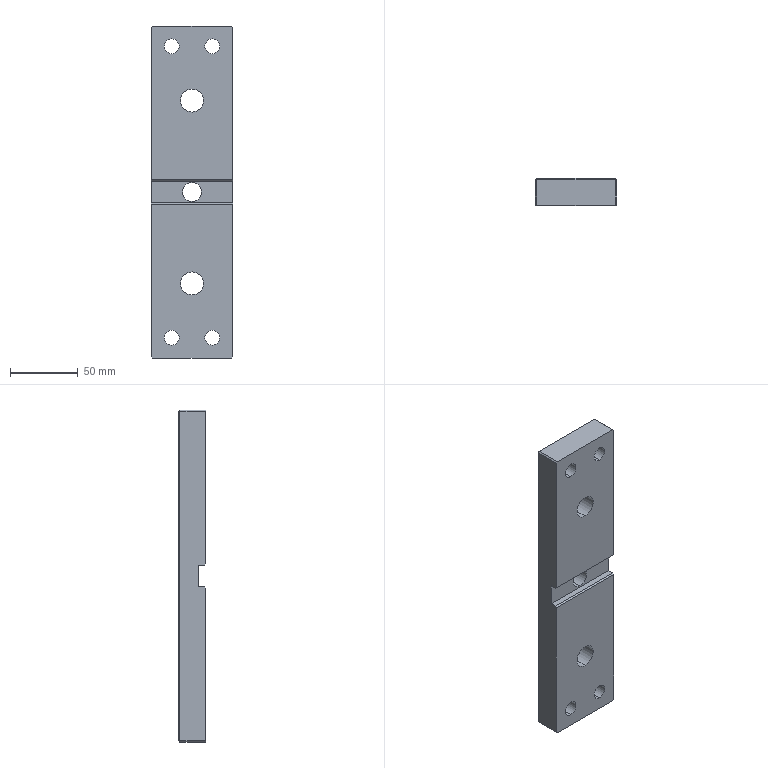Part | SolidWorks | features BaseBody 1 | 1 solid | 46 faces | box 60 x 20 x 245 mm | volume 258955 mm3 | plane 22 | cylinder 18 | cone 6 | commonest cylinder face diameters 11 x8 17 x4 40 x4 14 x2
STEP:
#1=CARTESIAN_POINT('',(15.,-10.,-113.));
#2=VERTEX_POINT('',#1);
#3=CARTESIAN_POINT('',(15.,-10.,-102.));
#4=VERTEX_POINT('',#3);
#5=CARTESIAN_POINT('',(15.,-10.,-107.5));
#6=DIRECTION('',(0.,1.,0.));
#7=DIRECTION('',(0.,0.,1.));
#8=AXIS2_PLACEMENT_3D('',#5,#6,#7);
#9=CIRCLE('',#8,5.5);
#10=EDGE_CURVE('',#2,#4,#9,.T.);
#11=ORIENTED_EDGE('',*,*,#10,.F.);
#12=CARTESIAN_POINT('',(15.,10.,-113.));
#13=VERTEX_POINT('',#12);
#14=CARTESIAN_POINT('',(15.,-10.,-113.));
#15=DIRECTION('',(0.,1.,0.));
#16=VECTOR('',#15,1000.);
#17=LINE('',#14,#16);
#18=EDGE_CURVE('',#2,#13,#17,.T.);
#19=ORIENTED_EDGE('',*,*,#18,.T.);
#20=CARTESIAN_POINT('',(15.,10.,-102.));
#21=VERTEX_POINT('',#20);
#22=CARTESIAN_POINT('',(15.,10.,-107.5));
#23=DIRECTION('',(0.,1.,0.));
#24=DIRECTION('',(0.,0.,1.));
#25=AXIS2_PLACEMENT_3D('',#22,#23,#24);
#26=CIRCLE('',#25,5.5);
#27=EDGE_CURVE('',#13,#21,#26,.T.);
#28=ORIENTED_EDGE('',*,*,#27,.T.);
#29=CARTESIAN_POINT('',(15.,-10.,-102.));
#30=DIRECTION('',(0.,1.,0.));
#31=VECTOR('',#30,1000.);
#32=LINE('',#29,#31);
#33=EDGE_CURVE('',#4,#21,#32,.T.);
#34=ORIENTED_EDGE('',*,*,#33,.F.);
#35=EDGE_LOOP('',(#11,#19,#28,#34));
#36=FACE_OUTER_BOUND('',#35,.T.);
#37=CARTESIAN_POINT('',(15.,-10.,-107.5));
#38=DIRECTION('',(0.,1.,0.));
#39=DIRECTION('',(0.,0.,1.));
#40=AXIS2_PLACEMENT_3D('',#37,#38,#39);
#41=CYLINDRICAL_SURFACE('',#40,5.5);
#42=ADVANCED_FACE('',(#36),#41,.F.);
#43=CARTESIAN_POINT('',(-15.,-10.,-113.));
#44=VERTEX_POINT('',#43);
#45=CARTESIAN_POINT('',(-15.,-10.,-102.));
#46=VERTEX_POINT('',#45);
#47=CARTESIAN_POINT('',(-15.,-10.,-107.5));
#48=DIRECTION('',(0.,1.,0.));
#49=DIRECTION('',(0.,0.,1.));
#50=AXIS2_PLACEMENT_3D('',#47,#48,#49);
#51=CIRCLE('',#50,5.5);
#52=EDGE_CURVE('',#44,#46,#51,.T.);
#53=ORIENTED_EDGE('',*,*,#52,.F.);
#54=CARTESIAN_POINT('',(-15.,10.,-113.));
#55=VERTEX_POINT('',#54);
#56=CARTESIAN_POINT('',(-15.,-10.,-113.));
#57=DIRECTION('',(0.,1.,0.));
#58=VECTOR('',#57,1000.);
#59=LINE('',#56,#58);
#60=EDGE_CURVE('',#44,#55,#59,.T.);
#61=ORIENTED_EDGE('',*,*,#60,.T.);
#62=CARTESIAN_POINT('',(-15.,10.,-102.));
#63=VERTEX_POINT('',#62);
#64=CARTESIAN_POINT('',(-15.,10.,-107.5));
#65=DIRECTION('',(0.,1.,0.));
#66=DIRECTION('',(0.,0.,1.));
#67=AXIS2_PLACEMENT_3D('',#64,#65,#66);
#68=CIRCLE('',#67,5.5);
#69=EDGE_CURVE('',#55,#63,#68,.T.);
#70=ORIENTED_EDGE('',*,*,#69,.T.);
#71=CARTESIAN_POINT('',(-15.,-10.,-102.));
#72=DIRECTION('',(0.,1.,0.));
#73=VECTOR('',#72,1000.);
#74=LINE('',#71,#73);
#75=EDGE_CURVE('',#46,#63,#74,.T.);
#76=ORIENTED_EDGE('',*,*,#75,.F.);
#77=EDGE_LOOP('',(#53,#61,#70,#76));
#78=FACE_OUTER_BOUND('',#77,.T.);
#79=CARTESIAN_POINT('',(-15.,-10.,-107.5));
#80=DIRECTION('',(0.,1.,0.));
#81=DIRECTION('',(0.,0.,1.));
#82=AXIS2_PLACEMENT_3D('',#79,#80,#81);
#83=CYLINDRICAL_SURFACE('',#82,5.5);
#84=ADVANCED_FACE('',(#78),#83,.F.);
#85=CARTESIAN_POINT('',(-15.,-10.,102.));
#86=VERTEX_POINT('',#85);
#87=CARTESIAN_POINT('',(-15.,-10.,113.));
#88=VERTEX_POINT('',#87);
#89=CARTESIAN_POINT('',(-15.,-10.,107.5));
#90=DIRECTION('',(0.,1.,0.));
#91=DIRECTION('',(0.,0.,1.));
#92=AXIS2_PLACEMENT_3D('',#89,#90,#91);
#93=CIRCLE('',#92,5.5);
#94=EDGE_CURVE('',#86,#88,#93,.T.);
#95=ORIENTED_EDGE('',*,*,#94,.F.);
#96=CARTESIAN_POINT('',(-15.,10.,102.));
#97=VERTEX_POINT('',#96);
#98=CARTESIAN_POINT('',(-15.,-10.,102.));
#99=DIRECTION('',(0.,1.,0.));
#100=VECTOR('',#99,1000.);
#101=LINE('',#98,#100);
#102=EDGE_CURVE('',#86,#97,#101,.T.);
#103=ORIENTED_EDGE('',*,*,#102,.T.);
#104=CARTESIAN_POINT('',(-15.,10.,113.));
#105=VERTEX_POINT('',#104);
#106=CARTESIAN_POINT('',(-15.,10.,107.5));
#107=DIRECTION('',(0.,1.,0.));
#108=DIRECTION('',(0.,0.,1.));
#109=AXIS2_PLACEMENT_3D('',#106,#107,#108);
#110=CIRCLE('',#109,5.5);
#111=EDGE_CURVE('',#97,#105,#110,.T.);
#112=ORIENTED_EDGE('',*,*,#111,.T.);
#113=CARTESIAN_POINT('',(-15.,-10.,113.));
#114=DIRECTION('',(0.,1.,0.));
#115=VECTOR('',#114,1000.);
#116=LINE('',#113,#115);
#117=EDGE_CURVE('',#88,#105,#116,.T.);
#118=ORIENTED_EDGE('',*,*,#117,.F.);
#119=EDGE_LOOP('',(#95,#103,#112,#118));
#120=FACE_OUTER_BOUND('',#119,.T.);
#121=CARTESIAN_POINT('',(-15.,-10.,107.5));
#122=DIRECTION('',(0.,1.,0.));
#123=DIRECTION('',(0.,0.,1.));
#124=AXIS2_PLACEMENT_3D('',#121,#122,#123);
#125=CYLINDRICAL_SURFACE('',#124,5.5);
#126=ADVANCED_FACE('',(#120),#125,.F.);
#127=CARTESIAN_POINT('',(15.,-10.,102.));
#128=VERTEX_POINT('',#127);
#129=CARTESIAN_POINT('',(15.,-10.,113.));
#130=VERTEX_POINT('',#129);
#131=CARTESIAN_POINT('',(15.,-10.,107.5));
#132=DIRECTION('',(0.,1.,0.));
#133=DIRECTION('',(0.,0.,1.));
#134=AXIS2_PLACEMENT_3D('',#131,#132,#133);
#135=CIRCLE('',#134,5.5);
#136=EDGE_CURVE('',#128,#130,#135,.T.);
#137=ORIENTED_EDGE('',*,*,#136,.F.);
#138=CARTESIAN_POINT('',(15.,10.,102.));
#139=VERTEX_POINT('',#138);
#140=CARTESIAN_POINT('',(15.,-10.,102.));
#141=DIRECTION('',(0.,1.,0.));
#142=VECTOR('',#141,1000.);
#143=LINE('',#140,#142);
#144=EDGE_CURVE('',#128,#139,#143,.T.);
#145=ORIENTED_EDGE('',*,*,#144,.T.);
#146=CARTESIAN_POINT('',(15.,10.,113.));
#147=VERTEX_POINT('',#146);
#148=CARTESIAN_POINT('',(15.,10.,107.5));
#149=DIRECTION('',(0.,1.,0.));
#150=DIRECTION('',(0.,0.,1.));
#151=AXIS2_PLACEMENT_3D('',#148,#149,#150);
#152=CIRCLE('',#151,5.5);
#153=EDGE_CURVE('',#139,#147,#152,.T.);
#154=ORIENTED_EDGE('',*,*,#153,.T.);
#155=CARTESIAN_POINT('',(15.,-10.,113.));
#156=DIRECTION('',(0.,1.,0.));
#157=VECTOR('',#156,1000.);
#158=LINE('',#155,#157);
#159=EDGE_CURVE('',#130,#147,#158,.T.);
#160=ORIENTED_EDGE('',*,*,#159,.F.);
#161=EDGE_LOOP('',(#137,#145,#154,#160));
#162=FACE_OUTER_BOUND('',#161,.T.);
#163=CARTESIAN_POINT('',(15.,-10.,107.5));
#164=DIRECTION('',(0.,1.,0.));
#165=DIRECTION('',(0.,0.,1.));
#166=AXIS2_PLACEMENT_3D('',#163,#164,#165);
#167=CYLINDRICAL_SURFACE('',#166,5.5);
#168=ADVANCED_FACE('',(#162),#167,.F.);
#169=CARTESIAN_POINT('',(0.,9.,-87.5));
#170=VERTEX_POINT('',#169);
#171=CARTESIAN_POINT('',(0.,9.,-47.5));
#172=VERTEX_POINT('',#171);
#173=CARTESIAN_POINT('',(0.,9.,-67.5));
#174=DIRECTION('',(0.,1.,0.));
#175=DIRECTION('',(0.,0.,-1.));
#176=AXIS2_PLACEMENT_3D('',#173,#174,#175);
#177=CIRCLE('',#176,20.);
#178=EDGE_CURVE('',#170,#172,#177,.T.);
#179=ORIENTED_EDGE('',*,*,#178,.F.);
#180=CARTESIAN_POINT('',(0.,10.,-88.5));
#181=VERTEX_POINT('',#180);
#182=CARTESIAN_POINT('',(0.,10.,-88.5));
#183=DIRECTION('',(0.,0.7071,-0.7071));
#184=VECTOR('',#183,1000.);
#185=LINE('',#182,#184);
#186=EDGE_CURVE('',#170,#181,#185,.T.);
#187=ORIENTED_EDGE('',*,*,#186,.T.);
#188=CARTESIAN_POINT('',(0.,10.,-46.5));
#189=VERTEX_POINT('',#188);
#190=CARTESIAN_POINT('',(0.,10.,-67.5));
#191=DIRECTION('',(0.,-1.,0.));
#192=DIRECTION('',(0.,0.,-1.));
#193=AXIS2_PLACEMENT_3D('',#190,#191,#192);
#194=CIRCLE('',#193,21.);
#195=EDGE_CURVE('',#189,#181,#194,.T.);
#196=ORIENTED_EDGE('',*,*,#195,.F.);
#197=CARTESIAN_POINT('',(0.,10.,-46.5));
#198=DIRECTION('',(0.,0.7071,0.7071));
#199=VECTOR('',#198,1000.);
#200=LINE('',#197,#199);
#201=EDGE_CURVE('',#172,#189,#200,.T.);
#202=ORIENTED_EDGE('',*,*,#201,.F.);
#203=EDGE_LOOP('',(#179,#187,#196,#202));
#204=FACE_OUTER_BOUND('',#203,.T.);
#205=CARTESIAN_POINT('',(0.,10.,-67.5));
#206=DIRECTION('',(0.,1.,0.));
#207=DIRECTION('',(0.,0.,1.));
#208=AXIS2_PLACEMENT_3D('',#205,#206,#207);
#209=CONICAL_SURFACE('',#208,21.,0.7854);
#210=ADVANCED_FACE('',(#204),#209,.F.);
#211=CARTESIAN_POINT('',(0.,9.,47.5));
#212=VERTEX_POINT('',#211);
#213=CARTESIAN_POINT('',(0.,9.,87.5));
#214=VERTEX_POINT('',#213);
#215=CARTESIAN_POINT('',(0.,9.,67.5));
#216=DIRECTION('',(0.,1.,0.));
#217=DIRECTION('',(0.,0.,-1.));
#218=AXIS2_PLACEMENT_3D('',#215,#216,#217);
#219=CIRCLE('',#218,20.);
#220=EDGE_CURVE('',#212,#214,#219,.T.);
#221=ORIENTED_EDGE('',*,*,#220,.F.);
#222=CARTESIAN_POINT('',(0.,10.,46.5));
#223=VERTEX_POINT('',#222);
#224=CARTESIAN_POINT('',(0.,10.,46.5));
#225=DIRECTION('',(0.,0.7071,-0.7071));
#226=VECTOR('',#225,1000.);
#227=LINE('',#224,#226);
#228=EDGE_CURVE('',#212,#223,#227,.T.);
#229=ORIENTED_EDGE('',*,*,#228,.T.);
#230=CARTESIAN_POINT('',(0.,10.,88.5));
#231=VERTEX_POINT('',#230);
#232=CARTESIAN_POINT('',(0.,10.,67.5));
#233=DIRECTION('',(0.,-1.,0.));
#234=DIRECTION('',(0.,0.,-1.));
#235=AXIS2_PLACEMENT_3D('',#232,#233,#234);
#236=CIRCLE('',#235,21.);
#237=EDGE_CURVE('',#231,#223,#236,.T.);
#238=ORIENTED_EDGE('',*,*,#237,.F.);
#239=CARTESIAN_POINT('',(0.,10.,88.5));
#240=DIRECTION('',(0.,0.7071,0.7071));
#241=VECTOR('',#240,1000.);
#242=LINE('',#239,#241);
#243=EDGE_CURVE('',#214,#231,#242,.T.);
#244=ORIENTED_EDGE('',*,*,#243,.F.);
#245=EDGE_LOOP('',(#221,#229,#238,#244));
#246=FACE_OUTER_BOUND('',#245,.T.);
#247=CARTESIAN_POINT('',(0.,10.,67.5));
#248=DIRECTION('',(0.,1.,0.));
#249=DIRECTION('',(0.,0.,1.));
#250=AXIS2_PLACEMENT_3D('',#247,#248,#249);
#251=CONICAL_SURFACE('',#250,21.,0.7854);
#252=ADVANCED_FACE('',(#246),#251,.F.);
#253=CARTESIAN_POINT('',(0.,8.975,-7.));
#254=VERTEX_POINT('',#253);
#255=CARTESIAN_POINT('',(0.,8.975,7.));
#256=VERTEX_POINT('',#255);
#257=CARTESIAN_POINT('',(0.,8.975,0.));
#258=DIRECTION('',(0.,1.,0.));
#259=DIRECTION('',(0.,0.,1.));
#260=AXIS2_PLACEMENT_3D('',#257,#258,#259);
#261=CIRCLE('',#260,7.);
#262=EDGE_CURVE('',#254,#256,#261,.T.);
#263=ORIENTED_EDGE('',*,*,#262,.F.);
#264=CARTESIAN_POINT('',(0.,10.,-8.025));
#265=VERTEX_POINT('',#264);
#266=CARTESIAN_POINT('',(0.,10.,-8.025));
#267=DIRECTION('',(0.,0.7071,-0.7071));
#268=VECTOR('',#267,1000.);
#269=LINE('',#266,#268);
#270=EDGE_CURVE('',#254,#265,#269,.T.);
#271=ORIENTED_EDGE('',*,*,#270,.T.);
#272=CARTESIAN_POINT('',(0.,10.,8.025));
#273=VERTEX_POINT('',#272);
#274=CARTESIAN_POINT('',(0.,10.,0.));
#275=DIRECTION('',(0.,1.,0.));
#276=DIRECTION('',(0.,0.,1.));
#277=AXIS2_PLACEMENT_3D('',#274,#275,#276);
#278=CIRCLE('',#277,8.025);
#279=EDGE_CURVE('',#265,#273,#278,.T.);
#280=ORIENTED_EDGE('',*,*,#279,.T.);
#281=CARTESIAN_POINT('',(0.,10.,8.025));
#282=DIRECTION('',(0.,0.7071,0.7071));
#283=VECTOR('',#282,1000.);
#284=LINE('',#281,#283);
#285=EDGE_CURVE('',#256,#273,#284,.T.);
#286=ORIENTED_EDGE('',*,*,#285,.F.);
#287=EDGE_LOOP('',(#263,#271,#280,#286));
#288=FACE_OUTER_BOUND('',#287,.T.);
#289=CARTESIAN_POINT('',(0.,10.,0.));
#290=DIRECTION('',(0.,1.,0.));
#291=DIRECTION('',(0.,0.,1.));
#292=AXIS2_PLACEMENT_3D('',#289,#290,#291);
#293=CONICAL_SURFACE('',#292,8.025,0.7854);
#294=ADVANCED_FACE('',(#288),#293,.F.);
#295=CARTESIAN_POINT('',(0.,-4.5,7.));
#296=VERTEX_POINT('',#295);
#297=CARTESIAN_POINT('',(0.,-4.5,-7.));
#298=VERTEX_POINT('',#297);
#299=CARTESIAN_POINT('',(0.,-4.5,0.));
#300=DIRECTION('',(0.,-1.,0.));
#301=DIRECTION('',(0.,0.,1.));
#302=AXIS2_PLACEMENT_3D('',#299,#300,#301);
#303=CIRCLE('',#302,7.);
#304=EDGE_CURVE('',#296,#298,#303,.T.);
#305=ORIENTED_EDGE('',*,*,#304,.T.);
#306=CARTESIAN_POINT('',(0.,10.,-7.));
#307=DIRECTION('',(0.,1.,0.));
#308=VECTOR('',#307,1000.);
#309=LINE('',#306,#308);
#310=EDGE_CURVE('',#298,#254,#309,.T.);
#311=ORIENTED_EDGE('',*,*,#310,.T.);
#312=ORIENTED_EDGE('',*,*,#262,.T.);
#313=CARTESIAN_POINT('',(0.,10.,7.));
#314=DIRECTION('',(0.,1.,0.));
#315=VECTOR('',#314,1000.);
#316=LINE('',#313,#315);
#317=EDGE_CURVE('',#296,#256,#316,.T.);
#318=ORIENTED_EDGE('',*,*,#317,.F.);
#319=EDGE_LOOP('',(#305,#311,#312,#318));
#320=FACE_OUTER_BOUND('',#319,.T.);
#321=CARTESIAN_POINT('',(0.,10.,0.));
#322=DIRECTION('',(0.,1.,0.));
#323=DIRECTION('',(0.,0.,1.));
#324=AXIS2_PLACEMENT_3D('',#321,#322,#323);
#325=CYLINDRICAL_SURFACE('',#324,7.);
#326=ADVANCED_FACE('',(#320),#325,.F.);
#327=CARTESIAN_POINT('',(0.,5.,87.5));
#328=VERTEX_POINT('',#327);
#329=CARTESIAN_POINT('',(0.,5.,47.5));
#330=VERTEX_POINT('',#329);
#331=CARTESIAN_POINT('',(0.,5.,67.5));
#332=DIRECTION('',(0.,-1.,0.));
#333=DIRECTION('',(0.,0.,-1.));
#334=AXIS2_PLACEMENT_3D('',#331,#332,#333);
#335=CIRCLE('',#334,20.);
#336=EDGE_CURVE('',#328,#330,#335,.T.);
#337=ORIENTED_EDGE('',*,*,#336,.T.);
#338=CARTESIAN_POINT('',(0.,5.,47.5));
#339=DIRECTION('',(0.,1.,0.));
#340=VECTOR('',#339,1000.);
#341=LINE('',#338,#340);
#342=EDGE_CURVE('',#330,#212,#341,.T.);
#343=ORIENTED_EDGE('',*,*,#342,.T.);
#344=ORIENTED_EDGE('',*,*,#220,.T.);
#345=CARTESIAN_POINT('',(0.,5.,87.5));
#346=DIRECTION('',(0.,1.,0.));
#347=VECTOR('',#346,1000.);
#348=LINE('',#345,#347);
#349=EDGE_CURVE('',#328,#214,#348,.T.);
#350=ORIENTED_EDGE('',*,*,#349,.F.);
#351=EDGE_LOOP('',(#337,#343,#344,#350));
#352=FACE_OUTER_BOUND('',#351,.T.);
#353=CARTESIAN_POINT('',(0.,5.,67.5));
#354=DIRECTION('',(0.,1.,0.));
#355=DIRECTION('',(0.,0.,1.));
#356=AXIS2_PLACEMENT_3D('',#353,#354,#355);
#357=CYLINDRICAL_SURFACE('',#356,20.);
#358=ADVANCED_FACE('',(#352),#357,.F.);
#359=CARTESIAN_POINT('',(0.,5.,-47.5));
#360=VERTEX_POINT('',#359);
#361=CARTESIAN_POINT('',(0.,5.,-87.5));
#362=VERTEX_POINT('',#361);
#363=CARTESIAN_POINT('',(0.,5.,-67.5));
#364=DIRECTION('',(0.,-1.,0.));
#365=DIRECTION('',(0.,0.,-1.));
#366=AXIS2_PLACEMENT_3D('',#363,#364,#365);
#367=CIRCLE('',#366,20.);
#368=EDGE_CURVE('',#360,#362,#367,.T.);
#369=ORIENTED_EDGE('',*,*,#368,.T.);
#370=CARTESIAN_POINT('',(0.,5.,-87.5));
#371=DIRECTION('',(0.,1.,0.));
#372=VECTOR('',#371,1000.);
#373=LINE('',#370,#372);
#374=EDGE_CURVE('',#362,#170,#373,.T.);
#375=ORIENTED_EDGE('',*,*,#374,.T.);
#376=ORIENTED_EDGE('',*,*,#178,.T.);
#377=CARTESIAN_POINT('',(0.,5.,-47.5));
#378=DIRECTION('',(0.,1.,0.));
#379=VECTOR('',#378,1000.);
#380=LINE('',#377,#379);
#381=EDGE_CURVE('',#360,#172,#380,.T.);
#382=ORIENTED_EDGE('',*,*,#381,.F.);
#383=EDGE_LOOP('',(#369,#375,#376,#382));
#384=FACE_OUTER_BOUND('',#383,.T.);
#385=CARTESIAN_POINT('',(0.,5.,-67.5));
#386=DIRECTION('',(0.,1.,0.));
#387=DIRECTION('',(0.,0.,1.));
#388=AXIS2_PLACEMENT_3D('',#385,#386,#387);
#389=CYLINDRICAL_SURFACE('',#388,20.);
#390=ADVANCED_FACE('',(#384),#389,.F.);
#391=CARTESIAN_POINT('',(0.,5.,-59.));
#392=VERTEX_POINT('',#391);
#393=CARTESIAN_POINT('',(0.,5.,-76.));
#394=VERTEX_POINT('',#393);
#395=CARTESIAN_POINT('',(0.,5.,-67.5));
#396=DIRECTION('',(0.,-1.,0.));
#397=DIRECTION('',(0.,0.,-1.));
#398=AXIS2_PLACEMENT_3D('',#395,#396,#397);
#399=CIRCLE('',#398,8.5);
#400=EDGE_CURVE('',#392,#394,#399,.T.);
#401=ORIENTED_EDGE('',*,*,#400,.F.);
#402=CARTESIAN_POINT('',(0.,-10.,-59.));
#403=VERTEX_POINT('',#402);
#404=CARTESIAN_POINT('',(0.,10.,-59.));
#405=DIRECTION('',(0.,-1.,0.));
#406=VECTOR('',#405,1000.);
#407=LINE('',#404,#406);
#408=EDGE_CURVE('',#392,#403,#407,.T.);
#409=ORIENTED_EDGE('',*,*,#408,.T.);
#410=CARTESIAN_POINT('',(0.,-10.,-76.));
#411=VERTEX_POINT('',#410);
#412=CARTESIAN_POINT('',(0.,-10.,-67.5));
#413=DIRECTION('',(0.,1.,0.));
#414=DIRECTION('',(0.,0.,1.));
#415=AXIS2_PLACEMENT_3D('',#412,#413,#414);
#416=CIRCLE('',#415,8.5);
#417=EDGE_CURVE('',#411,#403,#416,.T.);
#418=ORIENTED_EDGE('',*,*,#417,.F.);
#419=CARTESIAN_POINT('',(0.,10.,-76.));
#420=DIRECTION('',(0.,-1.,0.));
#421=VECTOR('',#420,1000.);
#422=LINE('',#419,#421);
#423=EDGE_CURVE('',#394,#411,#422,.T.);
#424=ORIENTED_EDGE('',*,*,#423,.F.);
#425=EDGE_LOOP('',(#401,#409,#418,#424));
#426=FACE_OUTER_BOUND('',#425,.T.);
#427=CARTESIAN_POINT('',(0.,10.,-67.5));
#428=DIRECTION('',(0.,-1.,0.));
#429=DIRECTION('',(0.,0.,-1.));
#430=AXIS2_PLACEMENT_3D('',#427,#428,#429);
#431=CYLINDRICAL_SURFACE('',#430,8.5);
#432=ADVANCED_FACE('',(#426),#431,.F.);
#433=CARTESIAN_POINT('',(0.,5.,76.));
#434=VERTEX_POINT('',#433);
#435=CARTESIAN_POINT('',(0.,5.,59.));
#436=VERTEX_POINT('',#435);
#437=CARTESIAN_POINT('',(0.,5.,67.5));
#438=DIRECTION('',(0.,-1.,0.));
#439=DIRECTION('',(0.,0.,-1.));
#440=AXIS2_PLACEMENT_3D('',#437,#438,#439);
#441=CIRCLE('',#440,8.5);
#442=EDGE_CURVE('',#434,#436,#441,.T.);
#443=ORIENTED_EDGE('',*,*,#442,.F.);
#444=CARTESIAN_POINT('',(0.,-10.,76.));
#445=VERTEX_POINT('',#444);
#446=CARTESIAN_POINT('',(0.,10.,76.));
#447=DIRECTION('',(0.,-1.,0.));
#448=VECTOR('',#447,1000.);
#449=LINE('',#446,#448);
#450=EDGE_CURVE('',#434,#445,#449,.T.);
#451=ORIENTED_EDGE('',*,*,#450,.T.);
#452=CARTESIAN_POINT('',(0.,-10.,59.));
#453=VERTEX_POINT('',#452);
#454=CARTESIAN_POINT('',(0.,-10.,67.5));
#455=DIRECTION('',(0.,1.,0.));
#456=DIRECTION('',(0.,0.,1.));
#457=AXIS2_PLACEMENT_3D('',#454,#455,#456);
#458=CIRCLE('',#457,8.5);
#459=EDGE_CURVE('',#453,#445,#458,.T.);
#460=ORIENTED_EDGE('',*,*,#459,.F.);
#461=CARTESIAN_POINT('',(0.,10.,59.));
#462=DIRECTION('',(0.,-1.,0.));
#463=VECTOR('',#462,1000.);
#464=LINE('',#461,#463);
#465=EDGE_CURVE('',#436,#453,#464,.T.);
#466=ORIENTED_EDGE('',*,*,#465,.F.);
#467=EDGE_LOOP('',(#443,#451,#460,#466));
#468=FACE_OUTER_BOUND('',#467,.T.);
#469=CARTESIAN_POINT('',(0.,10.,67.5));
#470=DIRECTION('',(0.,-1.,0.));
#471=DIRECTION('',(0.,0.,-1.));
#472=AXIS2_PLACEMENT_3D('',#469,#470,#471);
#473=CYLINDRICAL_SURFACE('',#472,8.5);
#474=ADVANCED_FACE('',(#468),#473,.F.);
#475=CARTESIAN_POINT('',(15.,-10.,-107.5));
#476=DIRECTION('',(0.,1.,0.));
#477=DIRECTION('',(0.,0.,1.));
#478=AXIS2_PLACEMENT_3D('',#475,#476,#477);
#479=CIRCLE('',#478,5.5);
#480=EDGE_CURVE('',#4,#2,#479,.T.);
#481=ORIENTED_EDGE('',*,*,#480,.T.);
#482=ORIENTED_EDGE('',*,*,#10,.T.);
#483=EDGE_LOOP('',(#481,#482));
#484=FACE_BOUND('',#483,.T.);
#485=CARTESIAN_POINT('',(-15.,-10.,-107.5));
#486=DIRECTION('',(0.,1.,0.));
#487=DIRECTION('',(0.,0.,1.));
#488=AXIS2_PLACEMENT_3D('',#485,#486,#487);
#489=CIRCLE('',#488,5.5);
#490=EDGE_CURVE('',#46,#44,#489,.T.);
#491=ORIENTED_EDGE('',*,*,#490,.T.);
#492=ORIENTED_EDGE('',*,*,#52,.T.);
#493=EDGE_LOOP('',(#491,#492));
#494=FACE_BOUND('',#493,.T.);
#495=CARTESIAN_POINT('',(30.,-10.,-9.));
#496=VERTEX_POINT('',#495);
#497=CARTESIAN_POINT('',(30.,-10.,-121.5));
#498=VERTEX_POINT('',#497);
#499=CARTESIAN_POINT('',(30.,-10.,-96.5));
#500=DIRECTION('',(0.,0.,-1.));
#501=VECTOR('',#500,1000.);
#502=LINE('',#499,#501);
#503=EDGE_CURVE('',#496,#498,#502,.T.);
#504=ORIENTED_EDGE('',*,*,#503,.F.);
#505=CARTESIAN_POINT('',(-30.,-10.,-9.));
#506=VERTEX_POINT('',#505);
#507=CARTESIAN_POINT('',(-30.,-10.,-9.));
#508=DIRECTION('',(-1.,0.,0.));
#509=VECTOR('',#508,1000.);
#510=LINE('',#507,#509);
#511=EDGE_CURVE('',#496,#506,#510,.T.);
#512=ORIENTED_EDGE('',*,*,#511,.T.);
#513=CARTESIAN_POINT('',(-30.,-10.,-121.5));
#514=VERTEX_POINT('',#513);
#515=CARTESIAN_POINT('',(-30.,-10.,96.5));
#516=DIRECTION('',(0.,0.,1.));
#517=VECTOR('',#516,1000.);
#518=LINE('',#515,#517);
#519=EDGE_CURVE('',#514,#506,#518,.T.);
#520=ORIENTED_EDGE('',*,*,#519,.F.);
#521=CARTESIAN_POINT('',(-29.,-10.,-122.5));
#522=VERTEX_POINT('',#521);
#523=CARTESIAN_POINT('',(-30.,-10.,-121.5));
#524=DIRECTION('',(-0.7071,0.,0.7071));
#525=VECTOR('',#524,1000.);
#526=LINE('',#523,#525);
#527=EDGE_CURVE('',#522,#514,#526,.T.);
#528=ORIENTED_EDGE('',*,*,#527,.F.);
#529=CARTESIAN_POINT('',(29.,-10.,-122.5));
#530=VERTEX_POINT('',#529);
#531=CARTESIAN_POINT('',(-29.,-10.,-122.5));
#532=DIRECTION('',(-1.,0.,0.));
#533=VECTOR('',#532,1000.);
#534=LINE('',#531,#533);
#535=EDGE_CURVE('',#530,#522,#534,.T.);
#536=ORIENTED_EDGE('',*,*,#535,.F.);
#537=CARTESIAN_POINT('',(29.,-10.,-122.5));
#538=DIRECTION('',(-0.7071,0.,-0.7071));
#539=VECTOR('',#538,1000.);
#540=LINE('',#537,#539);
#541=EDGE_CURVE('',#498,#530,#540,.T.);
#542=ORIENTED_EDGE('',*,*,#541,.F.);
#543=EDGE_LOOP('',(#504,#512,#520,#528,#536,#542));
#544=FACE_OUTER_BOUND('',#543,.T.);
#545=ORIENTED_EDGE('',*,*,#417,.T.);
#546=CARTESIAN_POINT('',(0.,-10.,-67.5));
#547=DIRECTION('',(0.,1.,0.));
#548=DIRECTION('',(0.,0.,1.));
#549=AXIS2_PLACEMENT_3D('',#546,#547,#548);
#550=CIRCLE('',#549,8.5);
#551=EDGE_CURVE('',#403,#411,#550,.T.);
#552=ORIENTED_EDGE('',*,*,#551,.T.);
#553=EDGE_LOOP('',(#545,#552));
#554=FACE_BOUND('',#553,.T.);
#555=CARTESIAN_POINT('',(0.,-10.,0.));
#556=DIRECTION('',(0.,-1.,0.));
#557=DIRECTION('',(0.,0.,-1.));
#558=AXIS2_PLACEMENT_3D('',#555,#556,#557);
#559=PLANE('',#558);
#560=ADVANCED_FACE('',(#484,#494,#544,#554),#559,.T.);
#561=CARTESIAN_POINT('',(-15.,10.,107.5));
#562=DIRECTION('',(0.,1.,0.));
#563=DIRECTION('',(0.,0.,1.));
#564=AXIS2_PLACEMENT_3D('',#561,#562,#563);
#565=CIRCLE('',#564,5.5);
#566=EDGE_CURVE('',#105,#97,#565,.T.);
#567=ORIENTED_EDGE('',*,*,#566,.F.);
#568=ORIENTED_EDGE('',*,*,#111,.F.);
#569=EDGE_LOOP('',(#567,#568));
#570=FACE_BOUND('',#569,.T.);
#571=CARTESIAN_POINT('',(15.,10.,107.5));
#572=DIRECTION('',(0.,1.,0.));
#573=DIRECTION('',(0.,0.,1.));
#574=AXIS2_PLACEMENT_3D('',#571,#572,#573);
#575=CIRCLE('',#574,5.5);
#576=EDGE_CURVE('',#147,#139,#575,.T.);
#577=ORIENTED_EDGE('',*,*,#576,.F.);
#578=ORIENTED_EDGE('',*,*,#153,.F.);
#579=EDGE_LOOP('',(#577,#578));
#580=FACE_BOUND('',#579,.T.);
#581=CARTESIAN_POINT('',(15.,10.,-107.5));
#582=DIRECTION('',(0.,1.,0.));
#583=DIRECTION('',(0.,0.,1.));
#584=AXIS2_PLACEMENT_3D('',#581,#582,#583);
#585=CIRCLE('',#584,5.5);
#586=EDGE_CURVE('',#21,#13,#585,.T.);
#587=ORIENTED_EDGE('',*,*,#586,.F.);
#588=ORIENTED_EDGE('',*,*,#27,.F.);
#589=EDGE_LOOP('',(#587,#588));
#590=FACE_BOUND('',#589,.T.);
#591=CARTESIAN_POINT('',(-15.,10.,-107.5));
#592=DIRECTION('',(0.,1.,0.));
#593=DIRECTION('',(0.,0.,1.));
#594=AXIS2_PLACEMENT_3D('',#591,#592,#593);
#595=CIRCLE('',#594,5.5);
#596=EDGE_CURVE('',#63,#55,#595,.T.);
#597=ORIENTED_EDGE('',*,*,#596,.F.);
#598=ORIENTED_EDGE('',*,*,#69,.F.);
#599=EDGE_LOOP('',(#597,#598));
#600=FACE_BOUND('',#599,.T.);
#601=ORIENTED_EDGE('',*,*,#237,.T.);
#602=CARTESIAN_POINT('',(0.,10.,67.5));
#603=DIRECTION('',(0.,-1.,0.));
#604=DIRECTION('',(0.,0.,-1.));
#605=AXIS2_PLACEMENT_3D('',#602,#603,#604);
#606=CIRCLE('',#605,21.);
#607=EDGE_CURVE('',#223,#231,#606,.T.);
#608=ORIENTED_EDGE('',*,*,#607,.T.);
#609=EDGE_LOOP('',(#601,#608));
#610=FACE_BOUND('',#609,.T.);
#611=ORIENTED_EDGE('',*,*,#195,.T.);
#612=CARTESIAN_POINT('',(0.,10.,-67.5));
#613=DIRECTION('',(0.,-1.,0.));
#614=DIRECTION('',(0.,0.,-1.));
#615=AXIS2_PLACEMENT_3D('',#612,#613,#614);
#616=CIRCLE('',#615,21.);
#617=EDGE_CURVE('',#181,#189,#616,.T.);
#618=ORIENTED_EDGE('',*,*,#617,.T.);
#619=EDGE_LOOP('',(#611,#618));
#620=FACE_BOUND('',#619,.T.);
#621=CARTESIAN_POINT('',(29.,10.,-121.5));
#622=VERTEX_POINT('',#621);
#623=CARTESIAN_POINT('',(-29.,10.,-121.5));
#624=VERTEX_POINT('',#623);
#625=CARTESIAN_POINT('',(0.,10.,-121.5));
#626=DIRECTION('',(-1.,0.,0.));
#627=VECTOR('',#626,1000.);
#628=LINE('',#625,#627);
#629=EDGE_CURVE('',#622,#624,#628,.T.);
#630=ORIENTED_EDGE('',*,*,#629,.T.);
#631=CARTESIAN_POINT('',(-29.,10.,121.5));
#632=VERTEX_POINT('',#631);
#633=CARTESIAN_POINT('',(-29.,10.,0.));
#634=DIRECTION('',(0.,0.,1.));
#635=VECTOR('',#634,1000.);
#636=LINE('',#633,#635);
#637=EDGE_CURVE('',#624,#632,#636,.T.);
#638=ORIENTED_EDGE('',*,*,#637,.T.);
#639=CARTESIAN_POINT('',(29.,10.,121.5));
#640=VERTEX_POINT('',#639);
#641=CARTESIAN_POINT('',(0.,10.,121.5));
#642=DIRECTION('',(1.,0.,0.));
#643=VECTOR('',#642,1000.);
#644=LINE('',#641,#643);
#645=EDGE_CURVE('',#632,#640,#644,.T.);
#646=ORIENTED_EDGE('',*,*,#645,.T.);
#647=CARTESIAN_POINT('',(29.,10.,0.));
#648=DIRECTION('',(0.,0.,-1.));
#649=VECTOR('',#648,1000.);
#650=LINE('',#647,#649);
#651=EDGE_CURVE('',#640,#622,#650,.T.);
#652=ORIENTED_EDGE('',*,*,#651,.T.);
#653=EDGE_LOOP('',(#630,#638,#646,#652));
#654=FACE_OUTER_BOUND('',#653,.T.);
#655=CARTESIAN_POINT('',(0.,10.,0.));
#656=DIRECTION('',(0.,1.,0.));
#657=DIRECTION('',(0.,0.,1.));
#658=AXIS2_PLACEMENT_3D('',#655,#656,#657);
#659=CIRCLE('',#658,8.025);
#660=EDGE_CURVE('',#273,#265,#659,.T.);
#661=ORIENTED_EDGE('',*,*,#660,.F.);
#662=ORIENTED_EDGE('',*,*,#279,.F.);
#663=EDGE_LOOP('',(#661,#662));
#664=FACE_BOUND('',#663,.T.);
#665=CARTESIAN_POINT('',(0.,10.,0.));
#666=DIRECTION('',(0.,-1.,0.));
#667=DIRECTION('',(0.,0.,-1.));
#668=AXIS2_PLACEMENT_3D('',#665,#666,#667);
#669=PLANE('',#668);
#670=ADVANCED_FACE('',(#570,#580,#590,#600,#610,#620,#654,#664),#669,.F.);
#671=CARTESIAN_POINT('',(-15.,-10.,107.5));
#672=DIRECTION('',(0.,1.,0.));
#673=DIRECTION('',(0.,0.,1.));
#674=AXIS2_PLACEMENT_3D('',#671,#672,#673);
#675=CIRCLE('',#674,5.5);
#676=EDGE_CURVE('',#88,#86,#675,.T.);
#677=ORIENTED_EDGE('',*,*,#676,.T.);
#678=ORIENTED_EDGE('',*,*,#94,.T.);
#679=EDGE_LOOP('',(#677,#678));
#680=FACE_BOUND('',#679,.T.);
#681=CARTESIAN_POINT('',(15.,-10.,107.5));
#682=DIRECTION('',(0.,1.,0.));
#683=DIRECTION('',(0.,0.,1.));
#684=AXIS2_PLACEMENT_3D('',#681,#682,#683);
#685=CIRCLE('',#684,5.5);
#686=EDGE_CURVE('',#130,#128,#685,.T.);
#687=ORIENTED_EDGE('',*,*,#686,.T.);
#688=ORIENTED_EDGE('',*,*,#136,.T.);
#689=EDGE_LOOP('',(#687,#688));
#690=FACE_BOUND('',#689,.T.);
#691=CARTESIAN_POINT('',(-30.,-10.,9.));
#692=VERTEX_POINT('',#691);
#693=CARTESIAN_POINT('',(-30.,-10.,121.5));
#694=VERTEX_POINT('',#693);
#695=CARTESIAN_POINT('',(-30.,-10.,96.5));
#696=DIRECTION('',(0.,0.,1.));
#697=VECTOR('',#696,1000.);
#698=LINE('',#695,#697);
#699=EDGE_CURVE('',#692,#694,#698,.T.);
#700=ORIENTED_EDGE('',*,*,#699,.F.);
#701=CARTESIAN_POINT('',(30.,-10.,9.));
#702=VERTEX_POINT('',#701);
#703=CARTESIAN_POINT('',(30.,-10.,9.));
#704=DIRECTION('',(1.,0.,0.));
#705=VECTOR('',#704,1000.);
#706=LINE('',#703,#705);
#707=EDGE_CURVE('',#692,#702,#706,.T.);
#708=ORIENTED_EDGE('',*,*,#707,.T.);
#709=CARTESIAN_POINT('',(30.,-10.,121.5));
#710=VERTEX_POINT('',#709);
#711=CARTESIAN_POINT('',(30.,-10.,-96.5));
#712=DIRECTION('',(0.,0.,-1.));
#713=VECTOR('',#712,1000.);
#714=LINE('',#711,#713);
#715=EDGE_CURVE('',#710,#702,#714,.T.);
#716=ORIENTED_EDGE('',*,*,#715,.F.);
#717=CARTESIAN_POINT('',(29.,-10.,122.5));
#718=VERTEX_POINT('',#717);
#719=CARTESIAN_POINT('',(30.,-10.,121.5));
#720=DIRECTION('',(0.7071,0.,-0.7071));
#721=VECTOR('',#720,1000.);
#722=LINE('',#719,#721);
#723=EDGE_CURVE('',#718,#710,#722,.T.);
#724=ORIENTED_EDGE('',*,*,#723,.F.);
#725=CARTESIAN_POINT('',(-29.,-10.,122.5));
#726=VERTEX_POINT('',#725);
#727=CARTESIAN_POINT('',(29.,-10.,122.5));
#728=DIRECTION('',(1.,0.,0.));
#729=VECTOR('',#728,1000.);
#730=LINE('',#727,#729);
#731=EDGE_CURVE('',#726,#718,#730,.T.);
#732=ORIENTED_EDGE('',*,*,#731,.F.);
#733=CARTESIAN_POINT('',(-29.,-10.,122.5));
#734=DIRECTION('',(0.7071,0.,0.7071));
#735=VECTOR('',#734,1000.);
#736=LINE('',#733,#735);
#737=EDGE_CURVE('',#694,#726,#736,.T.);
#738=ORIENTED_EDGE('',*,*,#737,.F.);
#739=EDGE_LOOP('',(#700,#708,#716,#724,#732,#738));
#740=FACE_OUTER_BOUND('',#739,.T.);
#741=ORIENTED_EDGE('',*,*,#459,.T.);
#742=CARTESIAN_POINT('',(0.,-10.,67.5));
#743=DIRECTION('',(0.,1.,0.));
#744=DIRECTION('',(0.,0.,1.));
#745=AXIS2_PLACEMENT_3D('',#742,#743,#744);
#746=CIRCLE('',#745,8.5);
#747=EDGE_CURVE('',#445,#453,#746,.T.);
#748=ORIENTED_EDGE('',*,*,#747,.T.);
#749=EDGE_LOOP('',(#741,#748));
#750=FACE_BOUND('',#749,.T.);
#751=CARTESIAN_POINT('',(0.,-10.,0.));
#752=DIRECTION('',(0.,-1.,0.));
#753=DIRECTION('',(0.,0.,-1.));
#754=AXIS2_PLACEMENT_3D('',#751,#752,#753);
#755=PLANE('',#754);
#756=ADVANCED_FACE('',(#680,#690,#740,#750),#755,.T.);
#757=CARTESIAN_POINT('',(-30.,9.,-121.5));
#758=VERTEX_POINT('',#757);
#759=CARTESIAN_POINT('',(-29.5,9.5,-122.));
#760=VERTEX_POINT('',#759);
#761=CARTESIAN_POINT('',(-61.5,-22.5,-90.));
#762=DIRECTION('',(0.5774,0.5774,-0.5774));
#763=VECTOR('',#762,1000.);
#764=LINE('',#761,#763);
#765=EDGE_CURVE('',#758,#760,#764,.T.);
#766=ORIENTED_EDGE('',*,*,#765,.T.);
#767=CARTESIAN_POINT('',(-29.,9.,-122.5));
#768=VERTEX_POINT('',#767);
#769=CARTESIAN_POINT('',(-20.,0.,-131.5));
#770=DIRECTION('',(0.5774,-0.5774,-0.5774));
#771=VECTOR('',#770,1000.);
#772=LINE('',#769,#771);
#773=EDGE_CURVE('',#760,#768,#772,.T.);
#774=ORIENTED_EDGE('',*,*,#773,.T.);
#775=CARTESIAN_POINT('',(-29.,10.,-122.5));
#776=DIRECTION('',(0.,-1.,0.));
#777=VECTOR('',#776,1000.);
#778=LINE('',#775,#777);
#779=EDGE_CURVE('',#768,#522,#778,.T.);
#780=ORIENTED_EDGE('',*,*,#779,.T.);
#781=ORIENTED_EDGE('',*,*,#527,.T.);
#782=CARTESIAN_POINT('',(-30.,10.,-121.5));
#783=DIRECTION('',(0.,-1.,0.));
#784=VECTOR('',#783,1000.);
#785=LINE('',#782,#784);
#786=EDGE_CURVE('',#758,#514,#785,.T.);
#787=ORIENTED_EDGE('',*,*,#786,.F.);
#788=EDGE_LOOP('',(#766,#774,#780,#781,#787));
#789=FACE_OUTER_BOUND('',#788,.T.);
#790=CARTESIAN_POINT('',(-30.,10.,-121.5));
#791=DIRECTION('',(0.7071,0.,0.7071));
#792=DIRECTION('',(0.7071,0.,-0.7071));
#793=AXIS2_PLACEMENT_3D('',#790,#791,#792);
#794=PLANE('',#793);
#795=ADVANCED_FACE('',(#789),#794,.F.);
#796=CARTESIAN_POINT('',(-30.,9.,121.5));
#797=VERTEX_POINT('',#796);
#798=CARTESIAN_POINT('',(-30.,10.,121.5));
#799=DIRECTION('',(0.,-1.,0.));
#800=VECTOR('',#799,1000.);
#801=LINE('',#798,#800);
#802=EDGE_CURVE('',#797,#694,#801,.T.);
#803=ORIENTED_EDGE('',*,*,#802,.F.);
#804=CARTESIAN_POINT('',(-30.,9.,96.5));
#805=DIRECTION('',(0.,0.,-1.));
#806=VECTOR('',#805,1000.);
#807=LINE('',#804,#806);
#808=EDGE_CURVE('',#797,#758,#807,.T.);
#809=ORIENTED_EDGE('',*,*,#808,.T.);
#810=ORIENTED_EDGE('',*,*,#786,.T.);
#811=ORIENTED_EDGE('',*,*,#519,.T.);
#812=CARTESIAN_POINT('',(-30.,-9.,-8.));
#813=VERTEX_POINT('',#812);
#814=CARTESIAN_POINT('',(-30.,-9.,-8.));
#815=DIRECTION('',(0.,0.7071,0.7071));
#816=VECTOR('',#815,1000.);
#817=LINE('',#814,#816);
#818=EDGE_CURVE('',#506,#813,#817,.T.);
#819=ORIENTED_EDGE('',*,*,#818,.T.);
#820=CARTESIAN_POINT('',(-30.,-4.5,-8.));
#821=VERTEX_POINT('',#820);
#822=CARTESIAN_POINT('',(-30.,-4.5,-8.));
#823=DIRECTION('',(0.,1.,0.));
#824=VECTOR('',#823,1000.);
#825=LINE('',#822,#824);
#826=EDGE_CURVE('',#813,#821,#825,.T.);
#827=ORIENTED_EDGE('',*,*,#826,.T.);
#828=CARTESIAN_POINT('',(-30.,-4.5,8.));
#829=VERTEX_POINT('',#828);
#830=CARTESIAN_POINT('',(-30.,-4.5,8.));
#831=DIRECTION('',(0.,0.,1.));
#832=VECTOR('',#831,1000.);
#833=LINE('',#830,#832);
#834=EDGE_CURVE('',#821,#829,#833,.T.);
#835=ORIENTED_EDGE('',*,*,#834,.T.);
#836=CARTESIAN_POINT('',(-30.,-9.,8.));
#837=VERTEX_POINT('',#836);
#838=CARTESIAN_POINT('',(-30.,-4.5,8.));
#839=DIRECTION('',(0.,-1.,0.));
#840=VECTOR('',#839,1000.);
#841=LINE('',#838,#840);
#842=EDGE_CURVE('',#829,#837,#841,.T.);
#843=ORIENTED_EDGE('',*,*,#842,.T.);
#844=CARTESIAN_POINT('',(-30.,-9.,8.));
#845=DIRECTION('',(0.,-0.7071,0.7071));
#846=VECTOR('',#845,1000.);
#847=LINE('',#844,#846);
#848=EDGE_CURVE('',#837,#692,#847,.T.);
#849=ORIENTED_EDGE('',*,*,#848,.T.);
#850=ORIENTED_EDGE('',*,*,#699,.T.);
#851=EDGE_LOOP('',(#803,#809,#810,#811,#819,#827,#835,#843,#849,#850));
#852=FACE_OUTER_BOUND('',#851,.T.);
#853=CARTESIAN_POINT('',(-30.,10.,96.5));
#854=DIRECTION('',(1.,0.,0.));
#855=DIRECTION('',(0.,0.,-1.));
#856=AXIS2_PLACEMENT_3D('',#853,#854,#855);
#857=PLANE('',#856);
#858=ADVANCED_FACE('',(#852),#857,.F.);
#859=CARTESIAN_POINT('',(-29.,9.,122.5));
#860=VERTEX_POINT('',#859);
#861=CARTESIAN_POINT('',(-29.,10.,122.5));
#862=DIRECTION('',(0.,-1.,0.));
#863=VECTOR('',#862,1000.);
#864=LINE('',#861,#863);
#865=EDGE_CURVE('',#860,#726,#864,.T.);
#866=ORIENTED_EDGE('',*,*,#865,.F.);
#867=CARTESIAN_POINT('',(-29.5,9.5,122.));
#868=VERTEX_POINT('',#867);
#869=CARTESIAN_POINT('',(-20.,0.,131.5));
#870=DIRECTION('',(-0.5774,0.5774,-0.5774));
#871=VECTOR('',#870,1000.);
#872=LINE('',#869,#871);
#873=EDGE_CURVE('',#860,#868,#872,.T.);
#874=ORIENTED_EDGE('',*,*,#873,.T.);
#875=CARTESIAN_POINT('',(-61.5,-22.5,90.));
#876=DIRECTION('',(-0.5774,-0.5774,-0.5774));
#877=VECTOR('',#876,1000.);
#878=LINE('',#875,#877);
#879=EDGE_CURVE('',#868,#797,#878,.T.);
#880=ORIENTED_EDGE('',*,*,#879,.T.);
#881=ORIENTED_EDGE('',*,*,#802,.T.);
#882=ORIENTED_EDGE('',*,*,#737,.T.);
#883=EDGE_LOOP('',(#866,#874,#880,#881,#882));
#884=FACE_OUTER_BOUND('',#883,.T.);
#885=CARTESIAN_POINT('',(-29.,10.,122.5));
#886=DIRECTION('',(0.7071,0.,-0.7071));
#887=DIRECTION('',(-0.7071,0.,-0.7071));
#888=AXIS2_PLACEMENT_3D('',#885,#886,#887);
#889=PLANE('',#888);
#890=ADVANCED_FACE('',(#884),#889,.F.);
#891=CARTESIAN_POINT('',(29.,9.,122.5));
#892=VERTEX_POINT('',#891);
#893=CARTESIAN_POINT('',(29.,10.,122.5));
#894=DIRECTION('',(0.,-1.,0.));
#895=VECTOR('',#894,1000.);
#896=LINE('',#893,#895);
#897=EDGE_CURVE('',#892,#718,#896,.T.);
#898=ORIENTED_EDGE('',*,*,#897,.F.);
#899=CARTESIAN_POINT('',(29.,9.,122.5));
#900=DIRECTION('',(-1.,0.,0.));
#901=VECTOR('',#900,1000.);
#902=LINE('',#899,#901);
#903=EDGE_CURVE('',#892,#860,#902,.T.);
#904=ORIENTED_EDGE('',*,*,#903,.T.);
#905=ORIENTED_EDGE('',*,*,#865,.T.);
#906=ORIENTED_EDGE('',*,*,#731,.T.);
#907=EDGE_LOOP('',(#898,#904,#905,#906));
#908=FACE_OUTER_BOUND('',#907,.T.);
#909=CARTESIAN_POINT('',(29.,10.,122.5));
#910=DIRECTION('',(0.,0.,-1.));
#911=DIRECTION('',(-1.,0.,0.));
#912=AXIS2_PLACEMENT_3D('',#909,#910,#911);
#913=PLANE('',#912);
#914=ADVANCED_FACE('',(#908),#913,.F.);
#915=CARTESIAN_POINT('',(30.,9.,121.5));
#916=VERTEX_POINT('',#915);
#917=CARTESIAN_POINT('',(29.5,9.5,122.));
#918=VERTEX_POINT('',#917);
#919=CARTESIAN_POINT('',(61.5,-22.5,90.));
#920=DIRECTION('',(-0.5774,0.5774,0.5774));
#921=VECTOR('',#920,1000.);
#922=LINE('',#919,#921);
#923=EDGE_CURVE('',#916,#918,#922,.T.);
#924=ORIENTED_EDGE('',*,*,#923,.T.);
#925=CARTESIAN_POINT('',(20.,0.,131.5));
#926=DIRECTION('',(-0.5774,-0.5774,0.5774));
#927=VECTOR('',#926,1000.);
#928=LINE('',#925,#927);
#929=EDGE_CURVE('',#918,#892,#928,.T.);
#930=ORIENTED_EDGE('',*,*,#929,.T.);
#931=ORIENTED_EDGE('',*,*,#897,.T.);
#932=ORIENTED_EDGE('',*,*,#723,.T.);
#933=CARTESIAN_POINT('',(30.,10.,121.5));
#934=DIRECTION('',(0.,-1.,0.));
#935=VECTOR('',#934,1000.);
#936=LINE('',#933,#935);
#937=EDGE_CURVE('',#916,#710,#936,.T.);
#938=ORIENTED_EDGE('',*,*,#937,.F.);
#939=EDGE_LOOP('',(#924,#930,#931,#932,#938));
#940=FACE_OUTER_BOUND('',#939,.T.);
#941=CARTESIAN_POINT('',(30.,10.,121.5));
#942=DIRECTION('',(-0.7071,0.,-0.7071));
#943=DIRECTION('',(-0.7071,0.,0.7071));
#944=AXIS2_PLACEMENT_3D('',#941,#942,#943);
#945=PLANE('',#944);
#946=ADVANCED_FACE('',(#940),#945,.F.);
#947=CARTESIAN_POINT('',(30.,9.,-121.5));
#948=VERTEX_POINT('',#947);
#949=CARTESIAN_POINT('',(30.,10.,-121.5));
#950=DIRECTION('',(0.,-1.,0.));
#951=VECTOR('',#950,1000.);
#952=LINE('',#949,#951);
#953=EDGE_CURVE('',#948,#498,#952,.T.);
#954=ORIENTED_EDGE('',*,*,#953,.F.);
#955=CARTESIAN_POINT('',(30.,9.,-96.5));
#956=DIRECTION('',(0.,0.,1.));
#957=VECTOR('',#956,1000.);
#958=LINE('',#955,#957);
#959=EDGE_CURVE('',#948,#916,#958,.T.);
#960=ORIENTED_EDGE('',*,*,#959,.T.);
#961=ORIENTED_EDGE('',*,*,#937,.T.);
#962=ORIENTED_EDGE('',*,*,#715,.T.);
#963=CARTESIAN_POINT('',(30.,-9.,8.));
#964=VERTEX_POINT('',#963);
#965=CARTESIAN_POINT('',(30.,-9.,8.));
#966=DIRECTION('',(0.,0.7071,-0.7071));
#967=VECTOR('',#966,1000.);
#968=LINE('',#965,#967);
#969=EDGE_CURVE('',#702,#964,#968,.T.);
#970=ORIENTED_EDGE('',*,*,#969,.T.);
#971=CARTESIAN_POINT('',(30.,-4.5,8.));
#972=VERTEX_POINT('',#971);
#973=CARTESIAN_POINT('',(30.,-4.5,8.));
#974=DIRECTION('',(0.,-1.,0.));
#975=VECTOR('',#974,1000.);
#976=LINE('',#973,#975);
#977=EDGE_CURVE('',#972,#964,#976,.T.);
#978=ORIENTED_EDGE('',*,*,#977,.F.);
#979=CARTESIAN_POINT('',(30.,-4.5,-8.));
#980=VERTEX_POINT('',#979);
#981=CARTESIAN_POINT('',(30.,-4.5,8.));
#982=DIRECTION('',(0.,0.,1.));
#983=VECTOR('',#982,1000.);
#984=LINE('',#981,#983);
#985=EDGE_CURVE('',#980,#972,#984,.T.);
#986=ORIENTED_EDGE('',*,*,#985,.F.);
#987=CARTESIAN_POINT('',(30.,-9.,-8.));
#988=VERTEX_POINT('',#987);
#989=CARTESIAN_POINT('',(30.,10.,-8.));
#990=DIRECTION('',(0.,-1.,0.));
#991=VECTOR('',#990,1000.);
#992=LINE('',#989,#991);
#993=EDGE_CURVE('',#980,#988,#992,.T.);
#994=ORIENTED_EDGE('',*,*,#993,.T.);
#995=CARTESIAN_POINT('',(30.,-9.,-8.));
#996=DIRECTION('',(0.,-0.7071,-0.7071));
#997=VECTOR('',#996,1000.);
#998=LINE('',#995,#997);
#999=EDGE_CURVE('',#988,#496,#998,.T.);
#1000=ORIENTED_EDGE('',*,*,#999,.T.);
#1001=ORIENTED_EDGE('',*,*,#503,.T.);
#1002=EDGE_LOOP('',(#954,#960,#961,#962,#970,#978,#986,#994,#1000,#1001));
#1003=FACE_OUTER_BOUND('',#1002,.T.);
#1004=CARTESIAN_POINT('',(30.,10.,-96.5));
#1005=DIRECTION('',(-1.,0.,0.));
#1006=DIRECTION('',(0.,0.,1.));
#1007=AXIS2_PLACEMENT_3D('',#1004,#1005,#1006);
#1008=PLANE('',#1007);
#1009=ADVANCED_FACE('',(#1003),#1008,.F.);
#1010=CARTESIAN_POINT('',(29.,9.,-122.5));
#1011=VERTEX_POINT('',#1010);
#1012=CARTESIAN_POINT('',(29.,10.,-122.5));
#1013=DIRECTION('',(0.,-1.,0.));
#1014=VECTOR('',#1013,1000.);
#1015=LINE('',#1012,#1014);
#1016=EDGE_CURVE('',#1011,#530,#1015,.T.);
#1017=ORIENTED_EDGE('',*,*,#1016,.F.);
#1018=CARTESIAN_POINT('',(29.5,9.5,-122.));
#1019=VERTEX_POINT('',#1018);
#1020=CARTESIAN_POINT('',(20.,0.,-131.5));
#1021=DIRECTION('',(0.5774,0.5774,0.5774));
#1022=VECTOR('',#1021,1000.);
#1023=LINE('',#1020,#1022);
#1024=EDGE_CURVE('',#1011,#1019,#1023,.T.);
#1025=ORIENTED_EDGE('',*,*,#1024,.T.);
#1026=CARTESIAN_POINT('',(61.5,-22.5,-90.));
#1027=DIRECTION('',(0.5774,-0.5774,0.5774));
#1028=VECTOR('',#1027,1000.);
#1029=LINE('',#1026,#1028);
#1030=EDGE_CURVE('',#1019,#948,#1029,.T.);
#1031=ORIENTED_EDGE('',*,*,#1030,.T.);
#1032=ORIENTED_EDGE('',*,*,#953,.T.);
#1033=ORIENTED_EDGE('',*,*,#541,.T.);
#1034=EDGE_LOOP('',(#1017,#1025,#1031,#1032,#1033));
#1035=FACE_OUTER_BOUND('',#1034,.T.);
#1036=CARTESIAN_POINT('',(29.,10.,-122.5));
#1037=DIRECTION('',(-0.7071,0.,0.7071));
#1038=DIRECTION('',(0.7071,0.,0.7071));
#1039=AXIS2_PLACEMENT_3D('',#1036,#1037,#1038);
#1040=PLANE('',#1039);
#1041=ADVANCED_FACE('',(#1035),#1040,.F.);
#1042=ORIENTED_EDGE('',*,*,#779,.F.);
#1043=CARTESIAN_POINT('',(-29.,9.,-122.5));
#1044=DIRECTION('',(1.,0.,0.));
#1045=VECTOR('',#1044,1000.);
#1046=LINE('',#1043,#1045);
#1047=EDGE_CURVE('',#768,#1011,#1046,.T.);
#1048=ORIENTED_EDGE('',*,*,#1047,.T.);
#1049=ORIENTED_EDGE('',*,*,#1016,.T.);
#1050=ORIENTED_EDGE('',*,*,#535,.T.);
#1051=EDGE_LOOP('',(#1042,#1048,#1049,#1050));
#1052=FACE_OUTER_BOUND('',#1051,.T.);
#1053=CARTESIAN_POINT('',(-29.,10.,-122.5));
#1054=DIRECTION('',(0.,0.,1.));
#1055=DIRECTION('',(1.,0.,0.));
#1056=AXIS2_PLACEMENT_3D('',#1053,#1054,#1055);
#1057=PLANE('',#1056);
#1058=ADVANCED_FACE('',(#1052),#1057,.F.);
#1059=ORIENTED_EDGE('',*,*,#450,.F.);
#1060=CARTESIAN_POINT('',(0.,5.,67.5));
#1061=DIRECTION('',(0.,-1.,0.));
#1062=DIRECTION('',(0.,0.,-1.));
#1063=AXIS2_PLACEMENT_3D('',#1060,#1061,#1062);
#1064=CIRCLE('',#1063,8.5);
#1065=EDGE_CURVE('',#436,#434,#1064,.T.);
#1066=ORIENTED_EDGE('',*,*,#1065,.F.);
#1067=ORIENTED_EDGE('',*,*,#465,.T.);
#1068=ORIENTED_EDGE('',*,*,#747,.F.);
#1069=EDGE_LOOP('',(#1059,#1066,#1067,#1068));
#1070=FACE_OUTER_BOUND('',#1069,.T.);
#1071=CARTESIAN_POINT('',(0.,10.,67.5));
#1072=DIRECTION('',(0.,-1.,0.));
#1073=DIRECTION('',(0.,0.,-1.));
#1074=AXIS2_PLACEMENT_3D('',#1071,#1072,#1073);
#1075=CYLINDRICAL_SURFACE('',#1074,8.5);
#1076=ADVANCED_FACE('',(#1070),#1075,.F.);
#1077=ORIENTED_EDGE('',*,*,#408,.F.);
#1078=CARTESIAN_POINT('',(0.,5.,-67.5));
#1079=DIRECTION('',(0.,-1.,0.));
#1080=DIRECTION('',(0.,0.,-1.));
#1081=AXIS2_PLACEMENT_3D('',#1078,#1079,#1080);
#1082=CIRCLE('',#1081,8.5);
#1083=EDGE_CURVE('',#394,#392,#1082,.T.);
#1084=ORIENTED_EDGE('',*,*,#1083,.F.);
#1085=ORIENTED_EDGE('',*,*,#423,.T.);
#1086=ORIENTED_EDGE('',*,*,#551,.F.);
#1087=EDGE_LOOP('',(#1077,#1084,#1085,#1086));
#1088=FACE_OUTER_BOUND('',#1087,.T.);
#1089=CARTESIAN_POINT('',(0.,10.,-67.5));
#1090=DIRECTION('',(0.,-1.,0.));
#1091=DIRECTION('',(0.,0.,-1.));
#1092=AXIS2_PLACEMENT_3D('',#1089,#1090,#1091);
#1093=CYLINDRICAL_SURFACE('',#1092,8.5);
#1094=ADVANCED_FACE('',(#1088),#1093,.F.);
#1095=ORIENTED_EDGE('',*,*,#374,.F.);
#1096=CARTESIAN_POINT('',(0.,5.,-67.5));
#1097=DIRECTION('',(0.,-1.,0.));
#1098=DIRECTION('',(0.,0.,-1.));
#1099=AXIS2_PLACEMENT_3D('',#1096,#1097,#1098);
#1100=CIRCLE('',#1099,20.);
#1101=EDGE_CURVE('',#362,#360,#1100,.T.);
#1102=ORIENTED_EDGE('',*,*,#1101,.T.);
#1103=ORIENTED_EDGE('',*,*,#381,.T.);
#1104=CARTESIAN_POINT('',(0.,9.,-67.5));
#1105=DIRECTION('',(0.,1.,0.));
#1106=DIRECTION('',(0.,0.,-1.));
#1107=AXIS2_PLACEMENT_3D('',#1104,#1105,#1106);
#1108=CIRCLE('',#1107,20.);
#1109=EDGE_CURVE('',#172,#170,#1108,.T.);
#1110=ORIENTED_EDGE('',*,*,#1109,.T.);
#1111=EDGE_LOOP('',(#1095,#1102,#1103,#1110));
#1112=FACE_OUTER_BOUND('',#1111,.T.);
#1113=CARTESIAN_POINT('',(0.,5.,-67.5));
#1114=DIRECTION('',(0.,1.,0.));
#1115=DIRECTION('',(0.,0.,1.));
#1116=AXIS2_PLACEMENT_3D('',#1113,#1114,#1115);
#1117=CYLINDRICAL_SURFACE('',#1116,20.);
#1118=ADVANCED_FACE('',(#1112),#1117,.F.);
#1119=ORIENTED_EDGE('',*,*,#1083,.T.);
#1120=ORIENTED_EDGE('',*,*,#400,.T.);
#1121=EDGE_LOOP('',(#1119,#1120));
#1122=FACE_BOUND('',#1121,.T.);
#1123=ORIENTED_EDGE('',*,*,#368,.F.);
#1124=ORIENTED_EDGE('',*,*,#1101,.F.);
#1125=EDGE_LOOP('',(#1123,#1124));
#1126=FACE_OUTER_BOUND('',#1125,.T.);
#1127=CARTESIAN_POINT('',(0.,5.,-67.5));
#1128=DIRECTION('',(0.,-1.,0.));
#1129=DIRECTION('',(0.,0.,-1.));
#1130=AXIS2_PLACEMENT_3D('',#1127,#1128,#1129);
#1131=PLANE('',#1130);
#1132=ADVANCED_FACE('',(#1122,#1126),#1131,.F.);
#1133=ORIENTED_EDGE('',*,*,#342,.F.);
#1134=CARTESIAN_POINT('',(0.,5.,67.5));
#1135=DIRECTION('',(0.,-1.,0.));
#1136=DIRECTION('',(0.,0.,-1.));
#1137=AXIS2_PLACEMENT_3D('',#1134,#1135,#1136);
#1138=CIRCLE('',#1137,20.);
#1139=EDGE_CURVE('',#330,#328,#1138,.T.);
#1140=ORIENTED_EDGE('',*,*,#1139,.T.);
#1141=ORIENTED_EDGE('',*,*,#349,.T.);
#1142=CARTESIAN_POINT('',(0.,9.,67.5));
#1143=DIRECTION('',(0.,1.,0.));
#1144=DIRECTION('',(0.,0.,-1.));
#1145=AXIS2_PLACEMENT_3D('',#1142,#1143,#1144);
#1146=CIRCLE('',#1145,20.);
#1147=EDGE_CURVE('',#214,#212,#1146,.T.);
#1148=ORIENTED_EDGE('',*,*,#1147,.T.);
#1149=EDGE_LOOP('',(#1133,#1140,#1141,#1148));
#1150=FACE_OUTER_BOUND('',#1149,.T.);
#1151=CARTESIAN_POINT('',(0.,5.,67.5));
#1152=DIRECTION('',(0.,1.,0.));
#1153=DIRECTION('',(0.,0.,1.));
#1154=AXIS2_PLACEMENT_3D('',#1151,#1152,#1153);
#1155=CYLINDRICAL_SURFACE('',#1154,20.);
#1156=ADVANCED_FACE('',(#1150),#1155,.F.);
#1157=ORIENTED_EDGE('',*,*,#1065,.T.);
#1158=ORIENTED_EDGE('',*,*,#442,.T.);
#1159=EDGE_LOOP('',(#1157,#1158));
#1160=FACE_BOUND('',#1159,.T.);
#1161=ORIENTED_EDGE('',*,*,#336,.F.);
#1162=ORIENTED_EDGE('',*,*,#1139,.F.);
#1163=EDGE_LOOP('',(#1161,#1162));
#1164=FACE_OUTER_BOUND('',#1163,.T.);
#1165=CARTESIAN_POINT('',(0.,5.,67.5));
#1166=DIRECTION('',(0.,-1.,0.));
#1167=DIRECTION('',(0.,0.,-1.));
#1168=AXIS2_PLACEMENT_3D('',#1165,#1166,#1167);
#1169=PLANE('',#1168);
#1170=ADVANCED_FACE('',(#1160,#1164),#1169,.F.);
#1171=ORIENTED_EDGE('',*,*,#310,.F.);
#1172=CARTESIAN_POINT('',(0.,-4.5,0.));
#1173=DIRECTION('',(0.,-1.,0.));
#1174=DIRECTION('',(0.,0.,1.));
#1175=AXIS2_PLACEMENT_3D('',#1172,#1173,#1174);
#1176=CIRCLE('',#1175,7.);
#1177=EDGE_CURVE('',#298,#296,#1176,.T.);
#1178=ORIENTED_EDGE('',*,*,#1177,.T.);
#1179=ORIENTED_EDGE('',*,*,#317,.T.);
#1180=CARTESIAN_POINT('',(0.,8.975,0.));
#1181=DIRECTION('',(0.,1.,0.));
#1182=DIRECTION('',(0.,0.,1.));
#1183=AXIS2_PLACEMENT_3D('',#1180,#1181,#1182);
#1184=CIRCLE('',#1183,7.);
#1185=EDGE_CURVE('',#256,#254,#1184,.T.);
#1186=ORIENTED_EDGE('',*,*,#1185,.T.);
#1187=EDGE_LOOP('',(#1171,#1178,#1179,#1186));
#1188=FACE_OUTER_BOUND('',#1187,.T.);
#1189=CARTESIAN_POINT('',(0.,10.,0.));
#1190=DIRECTION('',(0.,1.,0.));
#1191=DIRECTION('',(0.,0.,1.));
#1192=AXIS2_PLACEMENT_3D('',#1189,#1190,#1191);
#1193=CYLINDRICAL_SURFACE('',#1192,7.);
#1194=ADVANCED_FACE('',(#1188),#1193,.F.);
#1195=ORIENTED_EDGE('',*,*,#270,.F.);
#1196=ORIENTED_EDGE('',*,*,#1185,.F.);
#1197=ORIENTED_EDGE('',*,*,#285,.T.);
#1198=ORIENTED_EDGE('',*,*,#660,.T.);
#1199=EDGE_LOOP('',(#1195,#1196,#1197,#1198));
#1200=FACE_OUTER_BOUND('',#1199,.T.);
#1201=CARTESIAN_POINT('',(0.,10.,0.));
#1202=DIRECTION('',(0.,1.,0.));
#1203=DIRECTION('',(0.,0.,1.));
#1204=AXIS2_PLACEMENT_3D('',#1201,#1202,#1203);
#1205=CONICAL_SURFACE('',#1204,8.025,0.7854);
#1206=ADVANCED_FACE('',(#1200),#1205,.F.);
#1207=CARTESIAN_POINT('',(-30.,-4.5,8.));
#1208=DIRECTION('',(1.,0.,0.));
#1209=VECTOR('',#1208,1000.);
#1210=LINE('',#1207,#1209);
#1211=EDGE_CURVE('',#829,#972,#1210,.T.);
#1212=ORIENTED_EDGE('',*,*,#1211,.F.);
#1213=ORIENTED_EDGE('',*,*,#834,.F.);
#1214=CARTESIAN_POINT('',(-30.,-4.5,-8.));
#1215=DIRECTION('',(1.,0.,0.));
#1216=VECTOR('',#1215,1000.);
#1217=LINE('',#1214,#1216);
#1218=EDGE_CURVE('',#821,#980,#1217,.T.);
#1219=ORIENTED_EDGE('',*,*,#1218,.T.);
#1220=ORIENTED_EDGE('',*,*,#985,.T.);
#1221=EDGE_LOOP('',(#1212,#1213,#1219,#1220));
#1222=FACE_OUTER_BOUND('',#1221,.T.);
#1223=ORIENTED_EDGE('',*,*,#304,.F.);
#1224=ORIENTED_EDGE('',*,*,#1177,.F.);
#1225=EDGE_LOOP('',(#1223,#1224));
#1226=FACE_BOUND('',#1225,.T.);
#1227=CARTESIAN_POINT('',(-30.,-4.5,8.));
#1228=DIRECTION('',(0.,1.,0.));
#1229=DIRECTION('',(0.,0.,1.));
#1230=AXIS2_PLACEMENT_3D('',#1227,#1228,#1229);
#1231=PLANE('',#1230);
#1232=ADVANCED_FACE('',(#1222,#1226),#1231,.F.);
#1233=ORIENTED_EDGE('',*,*,#826,.F.);
#1234=CARTESIAN_POINT('',(30.,-9.,-8.));
#1235=DIRECTION('',(1.,0.,0.));
#1236=VECTOR('',#1235,1000.);
#1237=LINE('',#1234,#1236);
#1238=EDGE_CURVE('',#813,#988,#1237,.T.);
#1239=ORIENTED_EDGE('',*,*,#1238,.T.);
#1240=ORIENTED_EDGE('',*,*,#993,.F.);
#1241=ORIENTED_EDGE('',*,*,#1218,.F.);
#1242=EDGE_LOOP('',(#1233,#1239,#1240,#1241));
#1243=FACE_OUTER_BOUND('',#1242,.T.);
#1244=CARTESIAN_POINT('',(-30.,-4.5,-8.));
#1245=DIRECTION('',(0.,0.,-1.));
#1246=DIRECTION('',(-1.,0.,0.));
#1247=AXIS2_PLACEMENT_3D('',#1244,#1245,#1246);
#1248=PLANE('',#1247);
#1249=ADVANCED_FACE('',(#1243),#1248,.F.);
#1250=ORIENTED_EDGE('',*,*,#977,.T.);
#1251=CARTESIAN_POINT('',(-30.,-9.,8.));
#1252=DIRECTION('',(-1.,0.,0.));
#1253=VECTOR('',#1252,1000.);
#1254=LINE('',#1251,#1253);
#1255=EDGE_CURVE('',#964,#837,#1254,.T.);
#1256=ORIENTED_EDGE('',*,*,#1255,.T.);
#1257=ORIENTED_EDGE('',*,*,#842,.F.);
#1258=ORIENTED_EDGE('',*,*,#1211,.T.);
#1259=EDGE_LOOP('',(#1250,#1256,#1257,#1258));
#1260=FACE_OUTER_BOUND('',#1259,.T.);
#1261=CARTESIAN_POINT('',(-30.,-4.5,8.));
#1262=DIRECTION('',(0.,0.,1.));
#1263=DIRECTION('',(0.,-1.,0.));
#1264=AXIS2_PLACEMENT_3D('',#1261,#1262,#1263);
#1265=PLANE('',#1264);
#1266=ADVANCED_FACE('',(#1260),#1265,.F.);
#1267=ORIENTED_EDGE('',*,*,#228,.F.);
#1268=ORIENTED_EDGE('',*,*,#1147,.F.);
#1269=ORIENTED_EDGE('',*,*,#243,.T.);
#1270=ORIENTED_EDGE('',*,*,#607,.F.);
#1271=EDGE_LOOP('',(#1267,#1268,#1269,#1270));
#1272=FACE_OUTER_BOUND('',#1271,.T.);
#1273=CARTESIAN_POINT('',(0.,10.,67.5));
#1274=DIRECTION('',(0.,1.,0.));
#1275=DIRECTION('',(0.,0.,1.));
#1276=AXIS2_PLACEMENT_3D('',#1273,#1274,#1275);
#1277=CONICAL_SURFACE('',#1276,21.,0.7854);
#1278=ADVANCED_FACE('',(#1272),#1277,.F.);
#1279=ORIENTED_EDGE('',*,*,#186,.F.);
#1280=ORIENTED_EDGE('',*,*,#1109,.F.);
#1281=ORIENTED_EDGE('',*,*,#201,.T.);
#1282=ORIENTED_EDGE('',*,*,#617,.F.);
#1283=EDGE_LOOP('',(#1279,#1280,#1281,#1282));
#1284=FACE_OUTER_BOUND('',#1283,.T.);
#1285=CARTESIAN_POINT('',(0.,10.,-67.5));
#1286=DIRECTION('',(0.,1.,0.));
#1287=DIRECTION('',(0.,0.,1.));
#1288=AXIS2_PLACEMENT_3D('',#1285,#1286,#1287);
#1289=CONICAL_SURFACE('',#1288,21.,0.7854);
#1290=ADVANCED_FACE('',(#1284),#1289,.F.);
#1291=ORIENTED_EDGE('',*,*,#903,.F.);
#1292=ORIENTED_EDGE('',*,*,#929,.F.);
#1293=CARTESIAN_POINT('',(-3.167,42.167,89.333));
#1294=DIRECTION('',(0.5774,-0.5774,0.5774));
#1295=VECTOR('',#1294,1000.);
#1296=LINE('',#1293,#1295);
#1297=EDGE_CURVE('',#640,#918,#1296,.T.);
#1298=ORIENTED_EDGE('',*,*,#1297,.F.);
#1299=ORIENTED_EDGE('',*,*,#645,.F.);
#1300=CARTESIAN_POINT('',(-19.333,19.667,111.833));
#1301=DIRECTION('',(0.5774,0.5774,-0.5774));
#1302=VECTOR('',#1301,1000.);
#1303=LINE('',#1300,#1302);
#1304=EDGE_CURVE('',#868,#632,#1303,.T.);
#1305=ORIENTED_EDGE('',*,*,#1304,.F.);
#1306=ORIENTED_EDGE('',*,*,#873,.F.);
#1307=EDGE_LOOP('',(#1291,#1292,#1298,#1299,#1305,#1306));
#1308=FACE_OUTER_BOUND('',#1307,.T.);
#1309=CARTESIAN_POINT('',(0.,10.,121.5));
#1310=DIRECTION('',(0.,-0.7071,-0.7071));
#1311=DIRECTION('',(1.,0.,0.));
#1312=AXIS2_PLACEMENT_3D('',#1309,#1310,#1311);
#1313=PLANE('',#1312);
#1314=ADVANCED_FACE('',(#1308),#1313,.F.);
#1315=ORIENTED_EDGE('',*,*,#959,.F.);
#1316=ORIENTED_EDGE('',*,*,#1030,.F.);
#1317=CARTESIAN_POINT('',(19.333,19.667,-111.833));
#1318=DIRECTION('',(0.5774,-0.5774,-0.5774));
#1319=VECTOR('',#1318,1000.);
#1320=LINE('',#1317,#1319);
#1321=EDGE_CURVE('',#622,#1019,#1320,.T.);
#1322=ORIENTED_EDGE('',*,*,#1321,.F.);
#1323=ORIENTED_EDGE('',*,*,#651,.F.);
#1324=ORIENTED_EDGE('',*,*,#1297,.T.);
#1325=ORIENTED_EDGE('',*,*,#923,.F.);
#1326=EDGE_LOOP('',(#1315,#1316,#1322,#1323,#1324,#1325));
#1327=FACE_OUTER_BOUND('',#1326,.T.);
#1328=CARTESIAN_POINT('',(29.,10.,0.));
#1329=DIRECTION('',(-0.7071,-0.7071,0.));
#1330=DIRECTION('',(0.,0.,-1.));
#1331=AXIS2_PLACEMENT_3D('',#1328,#1329,#1330);
#1332=PLANE('',#1331);
#1333=ADVANCED_FACE('',(#1327),#1332,.F.);
#1334=ORIENTED_EDGE('',*,*,#1304,.T.);
#1335=ORIENTED_EDGE('',*,*,#637,.F.);
#1336=CARTESIAN_POINT('',(3.167,42.167,-89.333));
#1337=DIRECTION('',(0.5774,0.5774,0.5774));
#1338=VECTOR('',#1337,1000.);
#1339=LINE('',#1336,#1338);
#1340=EDGE_CURVE('',#760,#624,#1339,.T.);
#1341=ORIENTED_EDGE('',*,*,#1340,.F.);
#1342=ORIENTED_EDGE('',*,*,#765,.F.);
#1343=ORIENTED_EDGE('',*,*,#808,.F.);
#1344=ORIENTED_EDGE('',*,*,#879,.F.);
#1345=EDGE_LOOP('',(#1334,#1335,#1341,#1342,#1343,#1344));
#1346=FACE_OUTER_BOUND('',#1345,.T.);
#1347=CARTESIAN_POINT('',(-29.,10.,0.));
#1348=DIRECTION('',(0.7071,-0.7071,0.));
#1349=DIRECTION('',(0.,0.,1.));
#1350=AXIS2_PLACEMENT_3D('',#1347,#1348,#1349);
#1351=PLANE('',#1350);
#1352=ADVANCED_FACE('',(#1346),#1351,.F.);
#1353=ORIENTED_EDGE('',*,*,#1024,.F.);
#1354=ORIENTED_EDGE('',*,*,#1047,.F.);
#1355=ORIENTED_EDGE('',*,*,#773,.F.);
#1356=ORIENTED_EDGE('',*,*,#1340,.T.);
#1357=ORIENTED_EDGE('',*,*,#629,.F.);
#1358=ORIENTED_EDGE('',*,*,#1321,.T.);
#1359=EDGE_LOOP('',(#1353,#1354,#1355,#1356,#1357,#1358));
#1360=FACE_OUTER_BOUND('',#1359,.T.);
#1361=CARTESIAN_POINT('',(0.,10.,-121.5));
#1362=DIRECTION('',(0.,-0.7071,0.7071));
#1363=DIRECTION('',(-1.,0.,0.));
#1364=AXIS2_PLACEMENT_3D('',#1361,#1362,#1363);
#1365=PLANE('',#1364);
#1366=ADVANCED_FACE('',(#1360),#1365,.F.);
#1367=ORIENTED_EDGE('',*,*,#818,.F.);
#1368=ORIENTED_EDGE('',*,*,#511,.F.);
#1369=ORIENTED_EDGE('',*,*,#999,.F.);
#1370=ORIENTED_EDGE('',*,*,#1238,.F.);
#1371=EDGE_LOOP('',(#1367,#1368,#1369,#1370));
#1372=FACE_OUTER_BOUND('',#1371,.T.);
#1373=CARTESIAN_POINT('',(-30.,-9.,-8.));
#1374=DIRECTION('',(0.,-0.7071,0.7071));
#1375=DIRECTION('',(-1.,0.,0.));
#1376=AXIS2_PLACEMENT_3D('',#1373,#1374,#1375);
#1377=PLANE('',#1376);
#1378=ADVANCED_FACE('',(#1372),#1377,.T.);
#1379=ORIENTED_EDGE('',*,*,#969,.F.);
#1380=ORIENTED_EDGE('',*,*,#707,.F.);
#1381=ORIENTED_EDGE('',*,*,#848,.F.);
#1382=ORIENTED_EDGE('',*,*,#1255,.F.);
#1383=EDGE_LOOP('',(#1379,#1380,#1381,#1382));
#1384=FACE_OUTER_BOUND('',#1383,.T.);
#1385=CARTESIAN_POINT('',(-30.,-9.,8.));
#1386=DIRECTION('',(0.,-0.7071,-0.7071));
#1387=DIRECTION('',(1.,0.,0.));
#1388=AXIS2_PLACEMENT_3D('',#1385,#1386,#1387);
#1389=PLANE('',#1388);
#1390=ADVANCED_FACE('',(#1384),#1389,.T.);
#1391=ORIENTED_EDGE('',*,*,#144,.F.);
#1392=ORIENTED_EDGE('',*,*,#686,.F.);
#1393=ORIENTED_EDGE('',*,*,#159,.T.);
#1394=ORIENTED_EDGE('',*,*,#576,.T.);
#1395=EDGE_LOOP('',(#1391,#1392,#1393,#1394));
#1396=FACE_OUTER_BOUND('',#1395,.T.);
#1397=CARTESIAN_POINT('',(15.,-10.,107.5));
#1398=DIRECTION('',(0.,1.,0.));
#1399=DIRECTION('',(0.,0.,1.));
#1400=AXIS2_PLACEMENT_3D('',#1397,#1398,#1399);
#1401=CYLINDRICAL_SURFACE('',#1400,5.5);
#1402=ADVANCED_FACE('',(#1396),#1401,.F.);
#1403=ORIENTED_EDGE('',*,*,#102,.F.);
#1404=ORIENTED_EDGE('',*,*,#676,.F.);
#1405=ORIENTED_EDGE('',*,*,#117,.T.);
#1406=ORIENTED_EDGE('',*,*,#566,.T.);
#1407=EDGE_LOOP('',(#1403,#1404,#1405,#1406));
#1408=FACE_OUTER_BOUND('',#1407,.T.);
#1409=CARTESIAN_POINT('',(-15.,-10.,107.5));
#1410=DIRECTION('',(0.,1.,0.));
#1411=DIRECTION('',(0.,0.,1.));
#1412=AXIS2_PLACEMENT_3D('',#1409,#1410,#1411);
#1413=CYLINDRICAL_SURFACE('',#1412,5.5);
#1414=ADVANCED_FACE('',(#1408),#1413,.F.);
#1415=ORIENTED_EDGE('',*,*,#60,.F.);
#1416=ORIENTED_EDGE('',*,*,#490,.F.);
#1417=ORIENTED_EDGE('',*,*,#75,.T.);
#1418=ORIENTED_EDGE('',*,*,#596,.T.);
#1419=EDGE_LOOP('',(#1415,#1416,#1417,#1418));
#1420=FACE_OUTER_BOUND('',#1419,.T.);
#1421=CARTESIAN_POINT('',(-15.,-10.,-107.5));
#1422=DIRECTION('',(0.,1.,0.));
#1423=DIRECTION('',(0.,0.,1.));
#1424=AXIS2_PLACEMENT_3D('',#1421,#1422,#1423);
#1425=CYLINDRICAL_SURFACE('',#1424,5.5);
#1426=ADVANCED_FACE('',(#1420),#1425,.F.);
#1427=ORIENTED_EDGE('',*,*,#18,.F.);
#1428=ORIENTED_EDGE('',*,*,#480,.F.);
#1429=ORIENTED_EDGE('',*,*,#33,.T.);
#1430=ORIENTED_EDGE('',*,*,#586,.T.);
#1431=EDGE_LOOP('',(#1427,#1428,#1429,#1430));
#1432=FACE_OUTER_BOUND('',#1431,.T.);
#1433=CARTESIAN_POINT('',(15.,-10.,-107.5));
#1434=DIRECTION('',(0.,1.,0.));
#1435=DIRECTION('',(0.,0.,1.));
#1436=AXIS2_PLACEMENT_3D('',#1433,#1434,#1435);
#1437=CYLINDRICAL_SURFACE('',#1436,5.5);
#1438=ADVANCED_FACE('',(#1432),#1437,.F.);
#1439=CLOSED_SHELL('',(#42,#84,#126,#168,#210,#252,#294,#326,#358,#390,#432,#474,#560,#670,#756,#795,#858,#890,#914,#946,#1009,#1041,#1058,#1076,#1094,#1118,#1132,#1156,#1170,#1194,#1206,#1232,#1249,#1266,#1278,#1290,#1314,#1333,#1352,#1366,#1378,#1390,#1402,#1414,#1426,#1438));
#1440=MANIFOLD_SOLID_BREP('',#1439);
#1441=CARTESIAN_POINT('',(0.,0.,0.));
#1442=DIRECTION('',(0.,0.,1.));
#1443=DIRECTION('',(1.,0.,0.));
#1444=AXIS2_PLACEMENT_3D('',#1441,#1442,#1443);
#1445=(LENGTH_UNIT()NAMED_UNIT(*)SI_UNIT(.MILLI.,.METRE.));
#1446=UNCERTAINTY_MEASURE_WITH_UNIT(LENGTH_MEASURE(0.00001),#1445,'','');
#1447=(NAMED_UNIT(*)PLANE_ANGLE_UNIT()SI_UNIT($,.RADIAN.));
#1448=(NAMED_UNIT(*)SI_UNIT($,.STERADIAN.)SOLID_ANGLE_UNIT());
#1449=(GEOMETRIC_REPRESENTATION_CONTEXT(3)GLOBAL_UNCERTAINTY_ASSIGNED_CONTEXT((#1446))GLOBAL_UNIT_ASSIGNED_CONTEXT((#1445,#1447,#1448))REPRESENTATION_CONTEXT('',''));
#1450=ADVANCED_BREP_SHAPE_REPRESENTATION('',(#1440,#1444),#1449);